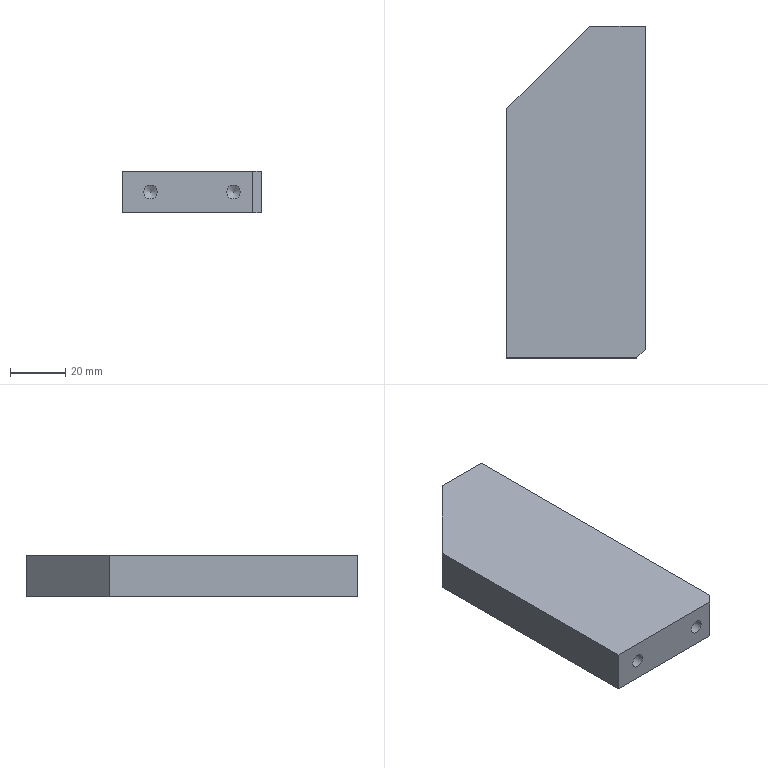Part | NX | 1 solid | 18 faces | box 50 x 120 x 15 mm | volume 81661 mm3 | plane 8 | cone 5 | cylinder 5 | commonest cylinder face diameters 5 x5
STEP:
#1=CARTESIAN_POINT('',(25.,8.,-2.5));
#2=VERTEX_POINT('',#1);
#3=CARTESIAN_POINT('',(25.,8.,0.));
#4=DIRECTION('',(1.,0.,0.));
#5=DIRECTION('',(0.,0.,-1.));
#6=AXIS2_PLACEMENT_3D('',#3,#4,#5);
#7=CIRCLE('',#6,2.5);
#8=EDGE_CURVE('',#2,#2,#7,.T.);
#9=ORIENTED_EDGE('',*,*,#8,.F.);
#10=EDGE_LOOP('',(#9));
#11=FACE_BOUND('',#10,.T.);
#12=CARTESIAN_POINT('',(25.,-32.,-2.5));
#13=VERTEX_POINT('',#12);
#14=CARTESIAN_POINT('',(25.,-32.,0.));
#15=DIRECTION('',(1.,0.,0.));
#16=DIRECTION('',(0.,0.,-1.));
#17=AXIS2_PLACEMENT_3D('',#14,#15,#16);
#18=CIRCLE('',#17,2.5);
#19=EDGE_CURVE('',#13,#13,#18,.T.);
#20=ORIENTED_EDGE('',*,*,#19,.F.);
#21=EDGE_LOOP('',(#20));
#22=FACE_BOUND('',#21,.T.);
#23=CARTESIAN_POINT('',(25.,-57.,7.5));
#24=VERTEX_POINT('',#23);
#25=CARTESIAN_POINT('',(25.,60.,7.5));
#26=VERTEX_POINT('',#25);
#27=CARTESIAN_POINT('',(25.,60.,7.5));
#28=DIRECTION('',(0.,1.,0.));
#29=VECTOR('',#28,1000.);
#30=LINE('',#27,#29);
#31=EDGE_CURVE('',#24,#26,#30,.T.);
#32=ORIENTED_EDGE('',*,*,#31,.F.);
#33=CARTESIAN_POINT('',(25.,-57.,-7.5));
#34=VERTEX_POINT('',#33);
#35=CARTESIAN_POINT('',(25.,-57.,7.5));
#36=DIRECTION('',(0.,0.,-1.));
#37=VECTOR('',#36,1000.);
#38=LINE('',#35,#37);
#39=EDGE_CURVE('',#24,#34,#38,.T.);
#40=ORIENTED_EDGE('',*,*,#39,.T.);
#41=CARTESIAN_POINT('',(25.,60.,-7.5));
#42=VERTEX_POINT('',#41);
#43=CARTESIAN_POINT('',(25.,60.,-7.5));
#44=DIRECTION('',(0.,1.,0.));
#45=VECTOR('',#44,1000.);
#46=LINE('',#43,#45);
#47=EDGE_CURVE('',#34,#42,#46,.T.);
#48=ORIENTED_EDGE('',*,*,#47,.T.);
#49=CARTESIAN_POINT('',(25.,60.,7.5));
#50=DIRECTION('',(0.,0.,-1.));
#51=VECTOR('',#50,1000.);
#52=LINE('',#49,#51);
#53=EDGE_CURVE('',#26,#42,#52,.T.);
#54=ORIENTED_EDGE('',*,*,#53,.F.);
#55=EDGE_LOOP('',(#32,#40,#48,#54));
#56=FACE_BOUND('',#55,.T.);
#57=CARTESIAN_POINT('',(25.,48.,-2.5));
#58=VERTEX_POINT('',#57);
#59=CARTESIAN_POINT('',(25.,48.,0.));
#60=DIRECTION('',(1.,0.,0.));
#61=DIRECTION('',(0.,0.,-1.));
#62=AXIS2_PLACEMENT_3D('',#59,#60,#61);
#63=CIRCLE('',#62,2.5);
#64=EDGE_CURVE('',#58,#58,#63,.T.);
#65=ORIENTED_EDGE('',*,*,#64,.F.);
#66=EDGE_LOOP('',(#65));
#67=FACE_BOUND('',#66,.T.);
#68=CARTESIAN_POINT('',(25.,60.,7.5));
#69=DIRECTION('',(-1.,0.,0.));
#70=DIRECTION('',(0.,-1.,0.));
#71=AXIS2_PLACEMENT_3D('',#68,#69,#70);
#72=PLANE('',#71);
#73=ADVANCED_FACE('',(#11,#22,#56,#67),#72,.F.);
#74=CARTESIAN_POINT('',(5.,60.,-7.5));
#75=VERTEX_POINT('',#74);
#76=CARTESIAN_POINT('',(-25.,60.,-7.5));
#77=DIRECTION('',(-1.,0.,0.));
#78=VECTOR('',#77,1000.);
#79=LINE('',#76,#78);
#80=EDGE_CURVE('',#42,#75,#79,.T.);
#81=ORIENTED_EDGE('',*,*,#80,.T.);
#82=CARTESIAN_POINT('',(5.,60.,7.5));
#83=VERTEX_POINT('',#82);
#84=CARTESIAN_POINT('',(5.,60.,7.5));
#85=DIRECTION('',(0.,0.,1.));
#86=VECTOR('',#85,1000.);
#87=LINE('',#84,#86);
#88=EDGE_CURVE('',#75,#83,#87,.T.);
#89=ORIENTED_EDGE('',*,*,#88,.T.);
#90=CARTESIAN_POINT('',(-25.,60.,7.5));
#91=DIRECTION('',(-1.,0.,0.));
#92=VECTOR('',#91,1000.);
#93=LINE('',#90,#92);
#94=EDGE_CURVE('',#26,#83,#93,.T.);
#95=ORIENTED_EDGE('',*,*,#94,.F.);
#96=ORIENTED_EDGE('',*,*,#53,.T.);
#97=EDGE_LOOP('',(#81,#89,#95,#96));
#98=FACE_BOUND('',#97,.T.);
#99=CARTESIAN_POINT('',(-25.,60.,7.5));
#100=DIRECTION('',(0.,-1.,0.));
#101=DIRECTION('',(0.,0.,-1.));
#102=AXIS2_PLACEMENT_3D('',#99,#100,#101);
#103=PLANE('',#102);
#104=ADVANCED_FACE('',(#98),#103,.F.);
#105=CARTESIAN_POINT('',(-25.,30.,7.5));
#106=VERTEX_POINT('',#105);
#107=CARTESIAN_POINT('',(-25.,-60.,7.5));
#108=VERTEX_POINT('',#107);
#109=CARTESIAN_POINT('',(-25.,60.,7.5));
#110=DIRECTION('',(0.,-1.,0.));
#111=VECTOR('',#110,1000.);
#112=LINE('',#109,#111);
#113=EDGE_CURVE('',#106,#108,#112,.T.);
#114=ORIENTED_EDGE('',*,*,#113,.F.);
#115=CARTESIAN_POINT('',(-25.,30.,-7.5));
#116=VERTEX_POINT('',#115);
#117=CARTESIAN_POINT('',(-25.,30.,7.5));
#118=DIRECTION('',(0.,0.,-1.));
#119=VECTOR('',#118,1000.);
#120=LINE('',#117,#119);
#121=EDGE_CURVE('',#106,#116,#120,.T.);
#122=ORIENTED_EDGE('',*,*,#121,.T.);
#123=CARTESIAN_POINT('',(-25.,-60.,-7.5));
#124=VERTEX_POINT('',#123);
#125=CARTESIAN_POINT('',(-25.,60.,-7.5));
#126=DIRECTION('',(0.,-1.,0.));
#127=VECTOR('',#126,1000.);
#128=LINE('',#125,#127);
#129=EDGE_CURVE('',#116,#124,#128,.T.);
#130=ORIENTED_EDGE('',*,*,#129,.T.);
#131=CARTESIAN_POINT('',(-25.,-60.,7.5));
#132=DIRECTION('',(0.,0.,-1.));
#133=VECTOR('',#132,1000.);
#134=LINE('',#131,#133);
#135=EDGE_CURVE('',#108,#124,#134,.T.);
#136=ORIENTED_EDGE('',*,*,#135,.F.);
#137=EDGE_LOOP('',(#114,#122,#130,#136));
#138=FACE_BOUND('',#137,.T.);
#139=CARTESIAN_POINT('',(-25.,60.,7.5));
#140=DIRECTION('',(1.,0.,0.));
#141=DIRECTION('',(0.,1.,0.));
#142=AXIS2_PLACEMENT_3D('',#139,#140,#141);
#143=PLANE('',#142);
#144=ADVANCED_FACE('',(#138),#143,.F.);
#145=CARTESIAN_POINT('',(-15.,-60.,-2.5));
#146=VERTEX_POINT('',#145);
#147=CARTESIAN_POINT('',(-15.,-60.,0.));
#148=DIRECTION('',(0.,-1.,0.));
#149=DIRECTION('',(0.,0.,-1.));
#150=AXIS2_PLACEMENT_3D('',#147,#148,#149);
#151=CIRCLE('',#150,2.5);
#152=EDGE_CURVE('',#146,#146,#151,.T.);
#153=ORIENTED_EDGE('',*,*,#152,.F.);
#154=EDGE_LOOP('',(#153));
#155=FACE_BOUND('',#154,.T.);
#156=CARTESIAN_POINT('',(15.,-60.,-2.5));
#157=VERTEX_POINT('',#156);
#158=CARTESIAN_POINT('',(15.,-60.,0.));
#159=DIRECTION('',(0.,-1.,0.));
#160=DIRECTION('',(0.,0.,-1.));
#161=AXIS2_PLACEMENT_3D('',#158,#159,#160);
#162=CIRCLE('',#161,2.5);
#163=EDGE_CURVE('',#157,#157,#162,.T.);
#164=ORIENTED_EDGE('',*,*,#163,.F.);
#165=EDGE_LOOP('',(#164));
#166=FACE_BOUND('',#165,.T.);
#167=CARTESIAN_POINT('',(22.,-60.,-7.5));
#168=VERTEX_POINT('',#167);
#169=CARTESIAN_POINT('',(-25.,-60.,-7.5));
#170=DIRECTION('',(1.,0.,0.));
#171=VECTOR('',#170,1000.);
#172=LINE('',#169,#171);
#173=EDGE_CURVE('',#124,#168,#172,.T.);
#174=ORIENTED_EDGE('',*,*,#173,.T.);
#175=CARTESIAN_POINT('',(22.,-60.,7.5));
#176=VERTEX_POINT('',#175);
#177=CARTESIAN_POINT('',(22.,-60.,7.5));
#178=DIRECTION('',(0.,0.,1.));
#179=VECTOR('',#178,1000.);
#180=LINE('',#177,#179);
#181=EDGE_CURVE('',#168,#176,#180,.T.);
#182=ORIENTED_EDGE('',*,*,#181,.T.);
#183=CARTESIAN_POINT('',(-25.,-60.,7.5));
#184=DIRECTION('',(1.,0.,0.));
#185=VECTOR('',#184,1000.);
#186=LINE('',#183,#185);
#187=EDGE_CURVE('',#108,#176,#186,.T.);
#188=ORIENTED_EDGE('',*,*,#187,.F.);
#189=ORIENTED_EDGE('',*,*,#135,.T.);
#190=EDGE_LOOP('',(#174,#182,#188,#189));
#191=FACE_BOUND('',#190,.T.);
#192=CARTESIAN_POINT('',(-25.,-60.,7.5));
#193=DIRECTION('',(0.,1.,0.));
#194=DIRECTION('',(0.,0.,1.));
#195=AXIS2_PLACEMENT_3D('',#192,#193,#194);
#196=PLANE('',#195);
#197=ADVANCED_FACE('',(#155,#166,#191),#196,.F.);
#198=ORIENTED_EDGE('',*,*,#187,.T.);
#199=CARTESIAN_POINT('',(41.,-41.,7.5));
#200=DIRECTION('',(-0.7071,-0.7071,0.));
#201=VECTOR('',#200,1000.);
#202=LINE('',#199,#201);
#203=EDGE_CURVE('',#176,#24,#202,.F.);
#204=ORIENTED_EDGE('',*,*,#203,.T.);
#205=ORIENTED_EDGE('',*,*,#31,.T.);
#206=ORIENTED_EDGE('',*,*,#94,.T.);
#207=CARTESIAN_POINT('',(-27.5,27.5,7.5));
#208=DIRECTION('',(0.7071,0.7071,0.));
#209=VECTOR('',#208,1000.);
#210=LINE('',#207,#209);
#211=EDGE_CURVE('',#83,#106,#210,.F.);
#212=ORIENTED_EDGE('',*,*,#211,.T.);
#213=ORIENTED_EDGE('',*,*,#113,.T.);
#214=EDGE_LOOP('',(#198,#204,#205,#206,#212,#213));
#215=FACE_BOUND('',#214,.T.);
#216=CARTESIAN_POINT('',(0.,0.,7.5));
#217=DIRECTION('',(0.,0.,1.));
#218=DIRECTION('',(1.,0.,0.));
#219=AXIS2_PLACEMENT_3D('',#216,#217,#218);
#220=PLANE('',#219);
#221=ADVANCED_FACE('',(#215),#220,.T.);
#222=ORIENTED_EDGE('',*,*,#47,.F.);
#223=CARTESIAN_POINT('',(25.,-57.,-7.5));
#224=DIRECTION('',(0.7071,0.7071,0.));
#225=VECTOR('',#224,1000.);
#226=LINE('',#223,#225);
#227=EDGE_CURVE('',#34,#168,#226,.F.);
#228=ORIENTED_EDGE('',*,*,#227,.T.);
#229=ORIENTED_EDGE('',*,*,#173,.F.);
#230=ORIENTED_EDGE('',*,*,#129,.F.);
#231=CARTESIAN_POINT('',(-25.,30.,-7.5));
#232=DIRECTION('',(-0.7071,-0.7071,0.));
#233=VECTOR('',#232,1000.);
#234=LINE('',#231,#233);
#235=EDGE_CURVE('',#116,#75,#234,.F.);
#236=ORIENTED_EDGE('',*,*,#235,.T.);
#237=ORIENTED_EDGE('',*,*,#80,.F.);
#238=EDGE_LOOP('',(#222,#228,#229,#230,#236,#237));
#239=FACE_BOUND('',#238,.T.);
#240=CARTESIAN_POINT('',(0.,0.,-7.5));
#241=DIRECTION('',(0.,0.,1.));
#242=DIRECTION('',(1.,0.,0.));
#243=AXIS2_PLACEMENT_3D('',#240,#241,#242);
#244=PLANE('',#243);
#245=ADVANCED_FACE('',(#239),#244,.F.);
#246=ORIENTED_EDGE('',*,*,#211,.F.);
#247=ORIENTED_EDGE('',*,*,#88,.F.);
#248=ORIENTED_EDGE('',*,*,#235,.F.);
#249=ORIENTED_EDGE('',*,*,#121,.F.);
#250=EDGE_LOOP('',(#246,#247,#248,#249));
#251=FACE_BOUND('',#250,.T.);
#252=CARTESIAN_POINT('',(-25.,30.,7.5));
#253=DIRECTION('',(0.7071,-0.7071,0.));
#254=DIRECTION('',(0.,0.,-1.));
#255=AXIS2_PLACEMENT_3D('',#252,#253,#254);
#256=PLANE('',#255);
#257=ADVANCED_FACE('',(#251),#256,.F.);
#258=CARTESIAN_POINT('',(8.498,-32.,0.));
#259=VERTEX_POINT('',#258);
#260=VERTEX_LOOP('',#259);
#261=FACE_BOUND('',#260,.T.);
#262=CARTESIAN_POINT('',(10.,-32.,-2.5));
#263=VERTEX_POINT('',#262);
#264=CARTESIAN_POINT('',(10.,-32.,0.));
#265=DIRECTION('',(1.,0.,0.));
#266=DIRECTION('',(0.,0.,-1.));
#267=AXIS2_PLACEMENT_3D('',#264,#265,#266);
#268=CIRCLE('',#267,2.5);
#269=EDGE_CURVE('',#263,#263,#268,.T.);
#270=ORIENTED_EDGE('',*,*,#269,.T.);
#271=EDGE_LOOP('',(#270));
#272=FACE_BOUND('',#271,.T.);
#273=CARTESIAN_POINT('',(10.,-32.,0.));
#274=DIRECTION('',(1.,0.,0.));
#275=DIRECTION('',(0.,0.,-1.));
#276=AXIS2_PLACEMENT_3D('',#273,#274,#275);
#277=CONICAL_SURFACE('',#276,2.5,1.03);
#278=ADVANCED_FACE('',(#261,#272),#277,.F.);
#279=ORIENTED_EDGE('',*,*,#269,.F.);
#280=EDGE_LOOP('',(#279));
#281=FACE_BOUND('',#280,.T.);
#282=ORIENTED_EDGE('',*,*,#19,.T.);
#283=EDGE_LOOP('',(#282));
#284=FACE_BOUND('',#283,.T.);
#285=CARTESIAN_POINT('',(25.,-32.,0.));
#286=DIRECTION('',(1.,0.,0.));
#287=DIRECTION('',(0.,0.,-1.));
#288=AXIS2_PLACEMENT_3D('',#285,#286,#287);
#289=CYLINDRICAL_SURFACE('',#288,2.5);
#290=ADVANCED_FACE('',(#281,#284),#289,.F.);
#291=CARTESIAN_POINT('',(15.,-43.498,0.));
#292=VERTEX_POINT('',#291);
#293=VERTEX_LOOP('',#292);
#294=FACE_BOUND('',#293,.T.);
#295=CARTESIAN_POINT('',(15.,-45.,-2.5));
#296=VERTEX_POINT('',#295);
#297=CARTESIAN_POINT('',(15.,-45.,0.));
#298=DIRECTION('',(0.,-1.,0.));
#299=DIRECTION('',(0.,0.,-1.));
#300=AXIS2_PLACEMENT_3D('',#297,#298,#299);
#301=CIRCLE('',#300,2.5);
#302=EDGE_CURVE('',#296,#296,#301,.T.);
#303=ORIENTED_EDGE('',*,*,#302,.T.);
#304=EDGE_LOOP('',(#303));
#305=FACE_BOUND('',#304,.T.);
#306=CARTESIAN_POINT('',(15.,-45.,0.));
#307=DIRECTION('',(0.,-1.,0.));
#308=DIRECTION('',(0.,0.,-1.));
#309=AXIS2_PLACEMENT_3D('',#306,#307,#308);
#310=CONICAL_SURFACE('',#309,2.5,1.03);
#311=ADVANCED_FACE('',(#294,#305),#310,.F.);
#312=ORIENTED_EDGE('',*,*,#302,.F.);
#313=EDGE_LOOP('',(#312));
#314=FACE_BOUND('',#313,.T.);
#315=ORIENTED_EDGE('',*,*,#163,.T.);
#316=EDGE_LOOP('',(#315));
#317=FACE_BOUND('',#316,.T.);
#318=CARTESIAN_POINT('',(15.,-60.,0.));
#319=DIRECTION('',(0.,-1.,0.));
#320=DIRECTION('',(0.,0.,-1.));
#321=AXIS2_PLACEMENT_3D('',#318,#319,#320);
#322=CYLINDRICAL_SURFACE('',#321,2.5);
#323=ADVANCED_FACE('',(#314,#317),#322,.F.);
#324=CARTESIAN_POINT('',(-15.,-43.498,0.));
#325=VERTEX_POINT('',#324);
#326=VERTEX_LOOP('',#325);
#327=FACE_BOUND('',#326,.T.);
#328=CARTESIAN_POINT('',(-15.,-45.,-2.5));
#329=VERTEX_POINT('',#328);
#330=CARTESIAN_POINT('',(-15.,-45.,0.));
#331=DIRECTION('',(0.,-1.,0.));
#332=DIRECTION('',(0.,0.,-1.));
#333=AXIS2_PLACEMENT_3D('',#330,#331,#332);
#334=CIRCLE('',#333,2.5);
#335=EDGE_CURVE('',#329,#329,#334,.T.);
#336=ORIENTED_EDGE('',*,*,#335,.T.);
#337=EDGE_LOOP('',(#336));
#338=FACE_BOUND('',#337,.T.);
#339=CARTESIAN_POINT('',(-15.,-45.,0.));
#340=DIRECTION('',(0.,-1.,0.));
#341=DIRECTION('',(0.,0.,-1.));
#342=AXIS2_PLACEMENT_3D('',#339,#340,#341);
#343=CONICAL_SURFACE('',#342,2.5,1.03);
#344=ADVANCED_FACE('',(#327,#338),#343,.F.);
#345=ORIENTED_EDGE('',*,*,#335,.F.);
#346=EDGE_LOOP('',(#345));
#347=FACE_BOUND('',#346,.T.);
#348=ORIENTED_EDGE('',*,*,#152,.T.);
#349=EDGE_LOOP('',(#348));
#350=FACE_BOUND('',#349,.T.);
#351=CARTESIAN_POINT('',(-15.,-60.,0.));
#352=DIRECTION('',(0.,-1.,0.));
#353=DIRECTION('',(0.,0.,-1.));
#354=AXIS2_PLACEMENT_3D('',#351,#352,#353);
#355=CYLINDRICAL_SURFACE('',#354,2.5);
#356=ADVANCED_FACE('',(#347,#350),#355,.F.);
#357=CARTESIAN_POINT('',(8.498,8.,0.));
#358=VERTEX_POINT('',#357);
#359=VERTEX_LOOP('',#358);
#360=FACE_BOUND('',#359,.T.);
#361=CARTESIAN_POINT('',(10.,8.,-2.5));
#362=VERTEX_POINT('',#361);
#363=CARTESIAN_POINT('',(10.,8.,0.));
#364=DIRECTION('',(1.,0.,0.));
#365=DIRECTION('',(0.,0.,-1.));
#366=AXIS2_PLACEMENT_3D('',#363,#364,#365);
#367=CIRCLE('',#366,2.5);
#368=EDGE_CURVE('',#362,#362,#367,.T.);
#369=ORIENTED_EDGE('',*,*,#368,.T.);
#370=EDGE_LOOP('',(#369));
#371=FACE_BOUND('',#370,.T.);
#372=CARTESIAN_POINT('',(10.,8.,0.));
#373=DIRECTION('',(1.,0.,0.));
#374=DIRECTION('',(0.,0.,-1.));
#375=AXIS2_PLACEMENT_3D('',#372,#373,#374);
#376=CONICAL_SURFACE('',#375,2.5,1.03);
#377=ADVANCED_FACE('',(#360,#371),#376,.F.);
#378=ORIENTED_EDGE('',*,*,#368,.F.);
#379=EDGE_LOOP('',(#378));
#380=FACE_BOUND('',#379,.T.);
#381=ORIENTED_EDGE('',*,*,#8,.T.);
#382=EDGE_LOOP('',(#381));
#383=FACE_BOUND('',#382,.T.);
#384=CARTESIAN_POINT('',(25.,8.,0.));
#385=DIRECTION('',(1.,0.,0.));
#386=DIRECTION('',(0.,0.,-1.));
#387=AXIS2_PLACEMENT_3D('',#384,#385,#386);
#388=CYLINDRICAL_SURFACE('',#387,2.5);
#389=ADVANCED_FACE('',(#380,#383),#388,.F.);
#390=CARTESIAN_POINT('',(10.,48.,-2.5));
#391=VERTEX_POINT('',#390);
#392=CARTESIAN_POINT('',(10.,48.,0.));
#393=DIRECTION('',(1.,0.,0.));
#394=DIRECTION('',(0.,0.,-1.));
#395=AXIS2_PLACEMENT_3D('',#392,#393,#394);
#396=CIRCLE('',#395,2.5);
#397=EDGE_CURVE('',#391,#391,#396,.T.);
#398=ORIENTED_EDGE('',*,*,#397,.F.);
#399=EDGE_LOOP('',(#398));
#400=FACE_BOUND('',#399,.T.);
#401=ORIENTED_EDGE('',*,*,#64,.T.);
#402=EDGE_LOOP('',(#401));
#403=FACE_BOUND('',#402,.T.);
#404=CARTESIAN_POINT('',(25.,48.,0.));
#405=DIRECTION('',(1.,0.,0.));
#406=DIRECTION('',(0.,0.,-1.));
#407=AXIS2_PLACEMENT_3D('',#404,#405,#406);
#408=CYLINDRICAL_SURFACE('',#407,2.5);
#409=ADVANCED_FACE('',(#400,#403),#408,.F.);
#410=CARTESIAN_POINT('',(8.498,48.,0.));
#411=VERTEX_POINT('',#410);
#412=VERTEX_LOOP('',#411);
#413=FACE_BOUND('',#412,.T.);
#414=ORIENTED_EDGE('',*,*,#397,.T.);
#415=EDGE_LOOP('',(#414));
#416=FACE_BOUND('',#415,.T.);
#417=CARTESIAN_POINT('',(10.,48.,0.));
#418=DIRECTION('',(1.,0.,0.));
#419=DIRECTION('',(0.,0.,-1.));
#420=AXIS2_PLACEMENT_3D('',#417,#418,#419);
#421=CONICAL_SURFACE('',#420,2.5,1.03);
#422=ADVANCED_FACE('',(#413,#416),#421,.F.);
#423=ORIENTED_EDGE('',*,*,#203,.F.);
#424=ORIENTED_EDGE('',*,*,#181,.F.);
#425=ORIENTED_EDGE('',*,*,#227,.F.);
#426=ORIENTED_EDGE('',*,*,#39,.F.);
#427=EDGE_LOOP('',(#423,#424,#425,#426));
#428=FACE_BOUND('',#427,.T.);
#429=CARTESIAN_POINT('',(25.,-57.,7.5));
#430=DIRECTION('',(-0.7071,0.7071,0.));
#431=DIRECTION('',(0.,0.,-1.));
#432=AXIS2_PLACEMENT_3D('',#429,#430,#431);
#433=PLANE('',#432);
#434=ADVANCED_FACE('',(#428),#433,.F.);
#435=CLOSED_SHELL('',(#73,#104,#144,#197,#221,#245,#257,#278,#290,#311,#323,#344,#356,#377,#389,#409,#422,#434));
#436=MANIFOLD_SOLID_BREP('',#435);
#437=(LENGTH_UNIT()NAMED_UNIT(*)SI_UNIT(.MILLI.,.METRE.));
#438=UNCERTAINTY_MEASURE_WITH_UNIT(LENGTH_MEASURE(0.00001),#437,'','');
#439=(NAMED_UNIT(*)PLANE_ANGLE_UNIT()SI_UNIT($,.RADIAN.));
#440=(NAMED_UNIT(*)SI_UNIT($,.STERADIAN.)SOLID_ANGLE_UNIT());
#441=(GEOMETRIC_REPRESENTATION_CONTEXT(3)GLOBAL_UNCERTAINTY_ASSIGNED_CONTEXT((#438))GLOBAL_UNIT_ASSIGNED_CONTEXT((#437,#439,#440))REPRESENTATION_CONTEXT('',''));
#442=ADVANCED_BREP_SHAPE_REPRESENTATION('',(#436),#441);